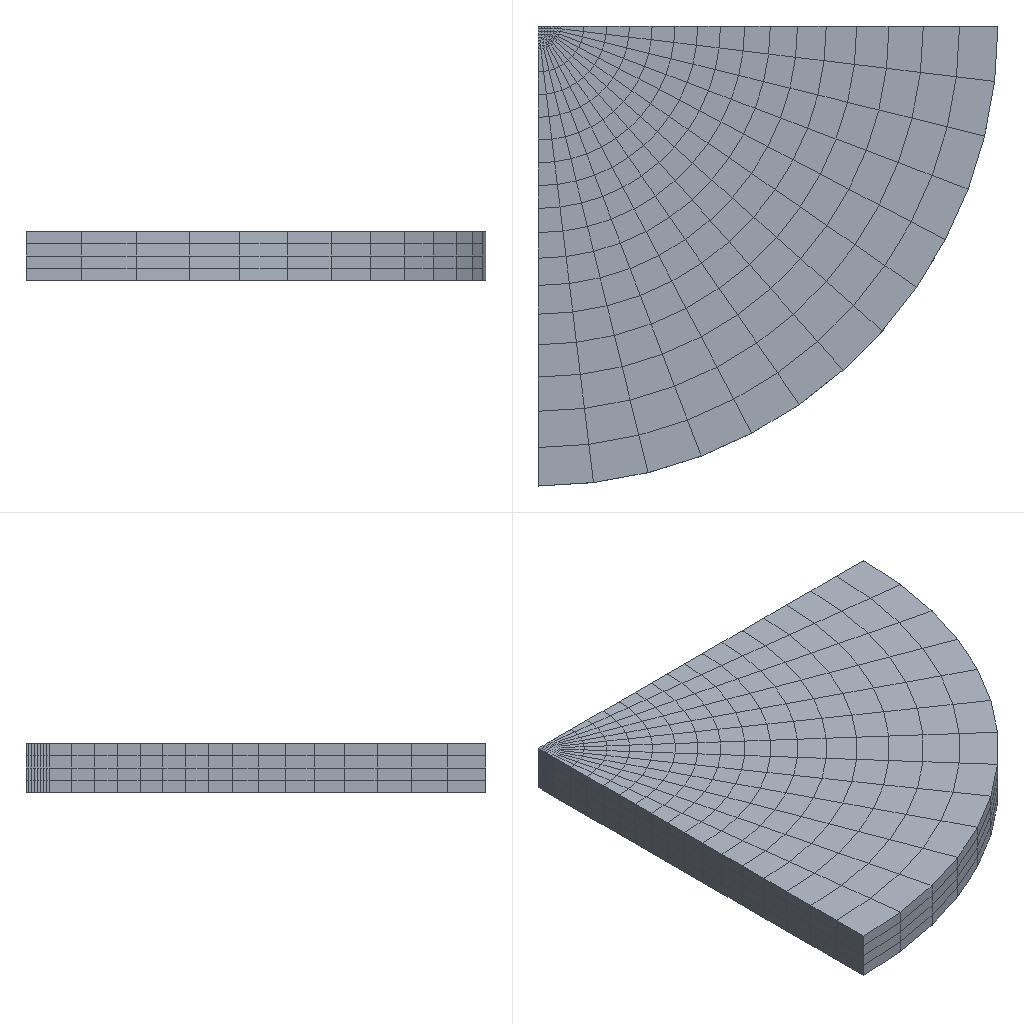Simulation study | abaqus
Set-up summary:
category,name,step,type,value,unit,region
solver,abaqus
solver,version,,,Abaqus/Standard 3DEXPERIENCE R2017x
units,not stated in the deck,,not stated
analysis,deck,,static,static
load_step,Step-1,Step-1,static
load_step,Step-2,Step-2,transient
load_step,requested,,,2
mesh,nodes,,,1795
mesh,elements,,,1319
element_type,R3D3,,rigid,4
element_type,R3D4,,rigid,263
element_type,C3D8R,,solid,1052
load,load commands in deck,,count,2
bc,support commands in deck,,count,19
material,MATERIAL-1,,in results
check,setup vs results,,match,"per instance, exact: element labels, types and connectivity; labels of the nodes the elements use; coordinates of those nodes at SINGLE_PRECISION in 2 of 4 instance(s)"
Abaqus input file, long lists of numbers shortened:
*Heading
** Job name: Job-2 Model name: Standard-Copy
** Generated by: Abaqus/CAE 2017
*Preprint, echo=NO, model=NO, history=NO, contact=NO
**
** PARTS
**
*Part, name=ball
*End Part
**
*Part, name=die
*End Part
**
*Part, name=holder
*End Part
**
*Part, name=specimen
*End Part
**
**
** ASSEMBLY
**
*Assembly, name=Assembly
**
*Instance, name=specimen-1, part=specimen
*Node
      1,           0., -0.2,           0.
      2,  0.2,           0.,           0.
** (1468 more lines like these left out)
*Element, type=C3D8R
  1,   88,  340,  841,  310,    1,   15,  190,   48
  2,  340,  341,  842,  841,   15,   16,  191,  190
** (1050 more lines like these left out)
*Nset, nset=Set-1, generate
    1,  1470,     1
*Elset, elset=Set-1, generate
    1,  1052,     1
*Nset, nset=Set-3, generate
    1,  1470,     1
*Elset, elset=Set-3, generate
    1,  1052,     1
*Elset, elset=_specimen-up_S1, internal
  235,  236,  237,  238,  239,  240,  241,  242,  243,  244,  245,  246,  247,  248,  249,  250
  251,  252,  253,  254,  255,  256,  257,  258,  259,  260,  261,  262,  263,  264,  265,  266
** (11 more lines like these left out)
*Elset, elset=_specimen-up_S3, internal
 423, 424, 425, 426, 427, 428, 449, 450, 451, 452, 453, 454, 455, 463, 464, 465
 466, 467, 468, 469, 477, 478, 479, 480, 481, 482, 483, 491, 492, 493, 494, 495
** (1 more lines like these left out)
*Elset, elset=_specimen-up_S4, internal, generate
 436,  448,    2
*Surface, type=ELEMENT, name=specimen-up
_specimen-up_S1, S1
_specimen-up_S3, S3
_specimen-up_S4, S4
*Elset, elset=_specimen-lower_S2, internal
   1,   2,   3,   4,   5,   6,   7,   8,   9,  10,  11,  12,  13,  14,  15,  16
  17,  18,  19,  20,  21,  22,  23,  24,  25,  26,  27,  28,  29,  30,  31,  32
** (15 more lines like these left out)
*Surface, type=ELEMENT, name=specimen-lower
_specimen-lower_S2, S2
*Orientation, name=Ori-10
          1.,           0.,           0.,           0.,           1.,           0.
1, 0.
** Section: Section-1
*Solid Section, elset=Set-3, orientation=Ori-10, material=Material-1
,
*End Instance
**
*Instance, name=die-1, part=die
 8.88178419700125e-16,           0.,           0.
 8.88178419700125e-16,           0.,           0.,           1.,           0.,           0.,          90.
*Node
      1,           0.,  -1.2,           2.
      2,           0., -0.2,           2.
** (152 more lines like these left out)
*Element, type=R3D4
 1,   1,   9,  71,  38
 2,   9,  10,  72,  71
** (128 more lines like these left out)
*Node
    155,    2.263,  1.09925615e-14,    2.263
*Nset, nset=die-1-RefPt_, internal
155,
*Elset, elset=_die_SPOS, internal, generate
   1,  130,    1
*Surface, type=ELEMENT, name=die
_die_SPOS, SPOS
*Elset, elset=die-1, generate
   1,  130,    1
*End Instance
**
*Instance, name=holder-1, part=holder
          0.,           0.,         0.42
          0.,           0.,         0.42,           1.,           0.,         0.42,          90.
*Node
      1,           0.,          1.5,         1.25
      2,           0.,           0.,         1.25
** (62 more lines like these left out)
*Element, type=R3D4
 1,  1,  7, 33, 16
 2,  7,  8, 34, 33
** (46 more lines like these left out)
*Element, type=R3D3
13, 57, 45, 43
*Node
     65,   2.298,  3.42011724e-15,   2.298
*Nset, nset=holder-1-RefPt_, internal
65,
*Elset, elset=_holder_SNEG, internal, generate
 13,  49,   1
*Surface, type=ELEMENT, name=holder
_holder_SNEG, SNEG
*Elset, elset=_hold-2_SNEG, internal, generate
  1,  12,   1
*Surface, type=ELEMENT, name=hold-2
_hold-2_SNEG, SNEG
*Elset, elset=holder-1, generate
  1,  49,   1
*End Instance
**
*Instance, name=ball-1, part=ball
          0.,  -8.32667268468867e-16,       -13.33
          0.,  -8.32667268468867e-16,       -13.33,           1.,  -8.32667268468867e-16,       -13.33,          90.
*Node
      1,           0.,    13.763,  0.1779
      2,           0.,   13.863,  0.5193
** (102 more lines like these left out)
*Element, type=R3D3
1, 75, 74, 71
2, 52, 51, 64
** (1 more lines like these left out)
*Element, type=R3D4
 4,  25,  24,   8,   1
 5,  78,  98,  77,  68
** (83 more lines like these left out)
*Node
    105,  7.6540425e-17,          15.,         1.25
*Nset, nset=ball-1-RefPt_, internal
105,
*Elset, elset=_ball_SNEG, internal, generate
  1,  88,   1
*Surface, type=ELEMENT, name=ball
_ball_SNEG, SNEG
*Elset, elset=ball-1, generate
  1,  88,   1
*End Instance
**
*Nset, nset=RP, instance=ball-1
 105,
*Nset, nset=Set-292, instance=ball-1
 105,
*Nset, nset=Set-293, instance=specimen-1
   2,   3,   5,   6,   9,  10,  11,  13,  27,  28,  29,  30,  31,  61,  62,  63
  64,  65,  89,  90,  91,  92,  93,  94,  95,  96,  97,  98,  99, 100, 108, 109
** (6 more lines like these left out)
*Elset, elset=Set-293, instance=specimen-1
   13,   26,   39,   52,   65,   78,   91,  104,  117,  130,  143,  156,  169,  182,  195,  208
  221,  234,  247,  260,  273,  286,  299,  312,  313,  320,  345,  352,  359,  366,  373,  380
** (4 more lines like these left out)
*Nset, nset=Set-294, instance=specimen-1
   1,   4,   7,   8,   9,  10,  12,  14,  44,  45,  46,  47,  48,  78,  79,  80
  81,  82,  83,  84,  85,  86,  87,  88, 101, 102, 103, 104, 105, 106, 107, 108
** (6 more lines like these left out)
*Elset, elset=Set-294, instance=specimen-1
    1,   14,   27,   40,   53,   66,   79,   92,  105,  118,  131,  144,  157,  170,  183,  196
  209,  222,  235,  248,  261,  274,  287,  300,  332,  338,  339,  340,  341,  342,  343,  344
** (4 more lines like these left out)
*Nset, nset=Set-295, instance=ball-1
 105,
*Nset, nset=Set-296, instance=die-1
 155,
*Nset, nset=Set-297, instance=holder-1
 65,
*Rigid Body, ref node=die-1.die-1-RefPt_, elset=die-1.die-1
*Rigid Body, ref node=holder-1.holder-1-RefPt_, elset=holder-1.holder-1
*Rigid Body, ref node=ball-1.ball-1-RefPt_, elset=ball-1.ball-1
*End Assembly
*Amplitude, name=Amp-2, time=TOTAL TIME
             0.,              0.,              1.,              1.
**
** MATERIALS
**
*Material, name=Material-1
*Creep
 4.8e-15, 5.75,   0.
*Potential
1.,1.,1.,1.,1.,1.
*Elastic
36000., 0.3
*Plastic
320.,0.
**
** INTERACTION PROPERTIES
**
*Surface Interaction, name=specimen_ball
1.,
*Friction, slip tolerance=0.005
 0.2,
*Surface Behavior, pressure-overclosure=HARD
*Surface Interaction, name=specimen_die
1.,
*Friction, slip tolerance=0.005
 0.2,
*Surface Behavior, pressure-overclosure=HARD
*Surface Interaction, name=specimen_holder
1.,
*Friction, slip tolerance=0.005
 0.2,
*Surface Behavior, pressure-overclosure=HARD
**
** BOUNDARY CONDITIONS
**
** Name: BC-5 Type: 对称/反对称/完全固定
*Boundary
Set-293, YSYMM
** Name: BC-7 Type: 对称/反对称/完全固定
*Boundary
Set-294, XSYMM
** Name: bc_ball_xz Type: Displacement/Rotation
*Boundary
Set-295, 1, 1
Set-295, 2, 2
Set-295, 4, 4
Set-295, 5, 5
Set-295, 6, 6
** Name: bc_die Type: Displacement/Rotation
*Boundary
Set-296, 1, 1
Set-296, 2, 2
Set-296, 3, 3
Set-296, 4, 4
Set-296, 5, 5
Set-296, 6, 6
** Name: bc_holder Type: Displacement/Rotation
*Boundary
Set-297, 1, 1
Set-297, 2, 2
Set-297, 3, 3
Set-297, 4, 4
Set-297, 5, 5
Set-297, 6, 6
**
** INTERACTIONS
**
** Interaction: Int-1
*Contact Pair, interaction=specimen_ball, type=SURFACE TO SURFACE, adjust=0.0
specimen-1.specimen-up, ball-1.ball
** Interaction: Int-2
*Contact Pair, interaction=specimen_holder, type=SURFACE TO SURFACE, adjust=0.0
specimen-1.specimen-up, holder-1.holder
** Interaction: Int-3
*Contact Pair, interaction=specimen_die, type=SURFACE TO SURFACE, adjust=0.0
specimen-1.specimen-lower, die-1.die
** ----------------------------------------------------------------
**
** STEP: Step-1
**
*Step, name=Step-1, nlgeom=YES, inc=1000
*Static, stabilize=0.0002, allsdtol=0.05, continue=NO
1e-08, 1e-06, 1e-11, 1e-06
**
** LOADS
**
** Name: Load-1   Type: Concentrated force
*Cload
Set-292, 2, 0.
Set-292, 3, -25.
**
** OUTPUT REQUESTS
**
*Restart, write, frequency=0
**
** FIELD OUTPUT: F-Output-1
**
*Output, field
*Node Output
CF, RF, RM, RT, U, V
*Element Output, directions=YES
E, LE, MISES, MISESMAX, MISESONLY, PE, PEEQ, PEEQT, PEMAG, S, SF, SSAVG, TSHR
*Contact Output
CDISP, CSTRESS
**
** HISTORY OUTPUT: H-Output-2
**
*Output, history
*Node Output, nset=RP
RF3, U3
**
** HISTORY OUTPUT: H-Output-1
**
*Output, history, variable=PRESELECT
*End Step
** ----------------------------------------------------------------
**
** STEP: Step-2
**
*Step, name=Step-2, nlgeom=YES, inc=5000
*Visco, cetol=1., creep=EXPLICIT, stabilize=0.0002, allsdtol=0.05, continue=NO
1., 1e+06, 1e-56, 1e+06
**
** CONTROLS
**
*Controls, reset
*Controls, parameters=time incrementation
, , , , , , , 50, , ,
**
** SOLVER CONTROLS
**
*Solver Controls, reset
*Solver Controls
,
**
** OUTPUT REQUESTS
**
*Restart, write, frequency=0
**
** FIELD OUTPUT: F-Output-1
**
*Output, field
*Node Output
CF, RF, U
*Element Output, directions=YES
CE, CEEQ, E, LE, PE, PEEQ, PEMAG, S
*Contact Output
CDISP, CSTRESS
**
** HISTORY OUTPUT: H-Output-2
**
*Output, history
*Node Output, nset=RP
RF3, U3
**
** HISTORY OUTPUT: H-Output-1
**
*Output, history, variable=PRESELECT
*End Step
Results summary:
result,step,,completed,increments=32 time=1e-06/1e-06
result,step,,partial,increments=192 time=8012.016/1000000.0
result,analysis,,,transient
result,last_loadstep,,,2
result,primary field,,,U
result,reaction total,,FX,0.000208,model units
result,reaction total,,FY,-0.00253,model units
result,reaction total,,FZ,24.945,model units